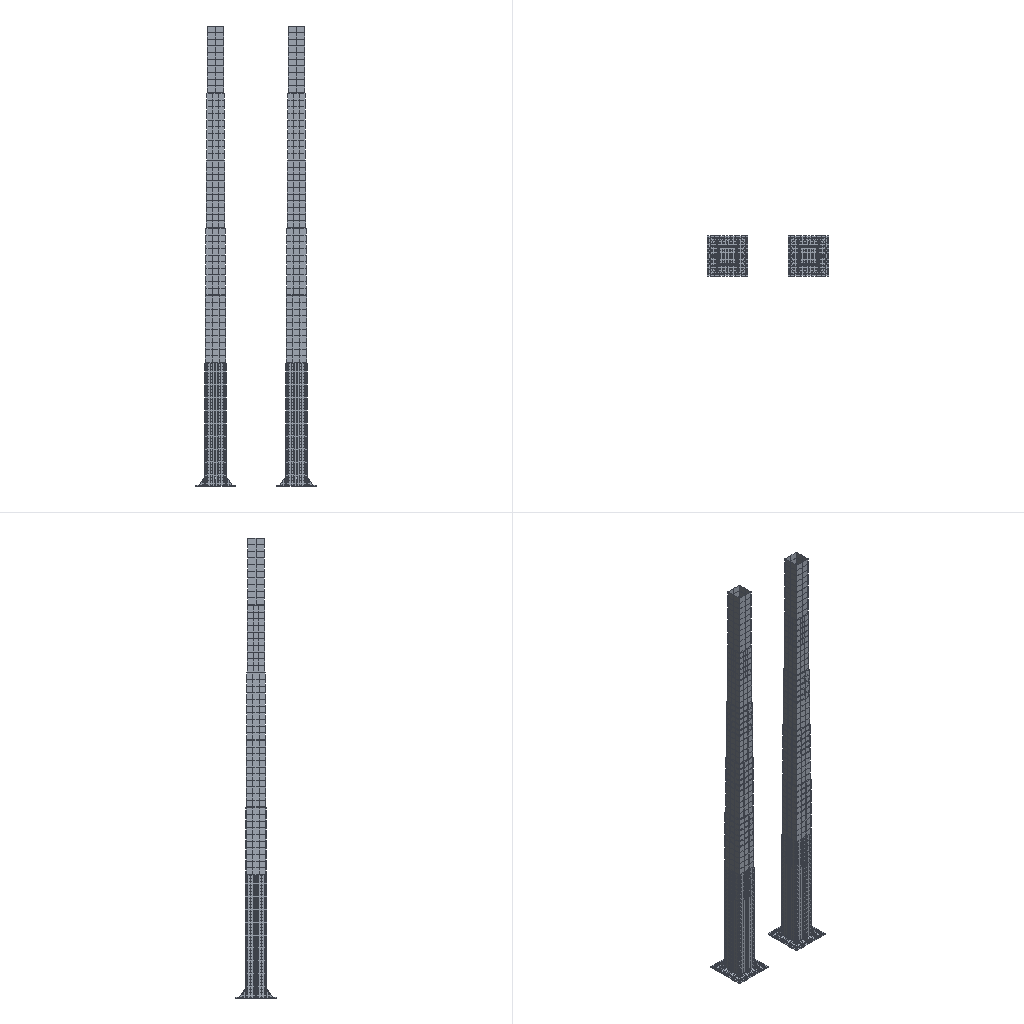Simulation study | abaqus
Set-up summary:
category,name,step,type,value,unit,region
solver,abaqus
solver,version,,,Abaqus/Standard 2020
units,not stated in the deck,,not stated
analysis,deck,,transient,transient
load_step,Step-1,Step-1,transient
load_step,requested,,,1
mesh,nodes,,,19952
mesh,elements,,,10428
element_type,C3D8R,,solid,10428
load,load commands in deck,,count,1
bc,support commands in deck,,count,1
material,MATERIAL-1,,in results
check,setup vs results,,match,"per instance, exact: element labels, types and connectivity; labels of the nodes the elements use; coordinates of those nodes at SINGLE_PRECISION in 12 of 12 instance(s)"
Abaqus input file, long lists of numbers shortened, first 444 of 2434 lines:
*Heading
** Job name: Job-1 Model name: Model-1
** Generated by: Abaqus/CAE 2020
*Preprint, echo=NO, model=NO, history=NO, contact=NO
**
** PARTS
**
*Part, name=work-1
*Node
      1,        -392.,         400.,   205.556
      2,        -400.,         400.,   205.556
** (8182 more lines like these left out)
*Element, type=C3D8R
 1,   11,    7,    8, 1147,    1,    2,    3,    4
 2, 1147,    8, 1146, 1148,    4,    3, 1079, 1078
** (4372 more lines like these left out)
*Nset, nset=Set-2, generate
    1,  8184,     1
*Elset, elset=Set-2, generate
    1,  4374,     1
** Section: Section-1
*Solid Section, elset=Set-2, material=Material-1
,
*End Part
**
*Part, name=work-2
*Node
      1,        381.5,        -379.,        3354.
      2,        381.5,         379.,        3354.
** (382 more lines like these left out)
*Element, type=C3D8R
  1,  22,  12,   1,   8,  46,  36,  25,  32
  2,  20,  14,   3,   7,  44,  38,  27,  31
** (178 more lines like these left out)
*Nset, nset=Set-1, generate
   1,  384,    1
*Elset, elset=Set-1, generate
   1,  180,    1
** Section: Section-1
*Solid Section, elset=Set-1, material=Material-1
,
*End Part
**
*Part, name=work-3
*Node
      1,        -305.,       -307.5,       13378.
      2,         305.,       -307.5,       13378.
** (254 more lines like these left out)
*Element, type=C3D8R
  1,  15,  10,   1,   8,  31,  26,  17,  24
  2,  14,  11,   3,   7,  30,  27,  19,  23
** (118 more lines like these left out)
*Nset, nset=Set-1, generate
   1,  256,    1
*Elset, elset=Set-1, generate
   1,  120,    1
** Section: Section-1
*Solid Section, elset=Set-1, material=Material-1
,
*End Part
**
*Part, name=work-4
*Node
      1,       -360.5,        -363.,        5860.
      2,        360.5,        -363.,        5860.
** (382 more lines like these left out)
*Element, type=C3D8R
  1,  22,  12,   1,   8,  46,  36,  25,  32
  2,  21,   7,   3,  11,  45,  31,  27,  35
** (178 more lines like these left out)
*Nset, nset=Set-1, generate
   1,  384,    1
*Elset, elset=Set-1, generate
   1,  180,    1
** Section: Section-1
*Solid Section, elset=Set-1, material=Material-1
,
*End Part
**
*Part, name=work-5
*Node
      1,        -342.,       -344.5,        8366.
      2,         342.,       -344.5,        8366.
** (382 more lines like these left out)
*Element, type=C3D8R
  1,  22,  12,   1,   8,  46,  36,  25,  32
  2,  21,   7,   3,  11,  45,  31,  27,  35
** (178 more lines like these left out)
*Nset, nset=Set-1, generate
   1,  384,    1
*Elset, elset=Set-1, generate
   1,  180,    1
** Section: Section-1
*Solid Section, elset=Set-1, material=Material-1
,
*End Part
**
*Part, name=work-6
*Node
      1,        323.5,        -326.,       10872.
      2,        323.5,         326.,       10872.
** (382 more lines like these left out)
*Element, type=C3D8R
  1,  22,  12,   1,   8,  46,  36,  25,  32
  2,  20,  14,   3,   7,  44,  38,  27,  31
** (178 more lines like these left out)
*Nset, nset=Set-1, generate
   1,  384,    1
*Elset, elset=Set-1, generate
   1,  180,    1
** Section: Section-1
*Solid Section, elset=Set-1, material=Material-1
,
*End Part
**
*Part, name=work-8
*Node
      1,        3342.,       -344.5,       12073.
      2,        2658.,       -344.5,       12073.
** (382 more lines like these left out)
*Element, type=C3D8R
  1,  22,  12,   1,   8,  46,  36,  25,  32
  2,  20,  14,   3,   7,  44,  38,  27,  31
** (178 more lines like these left out)
*Nset, nset=Set-1, generate
   1,  384,    1
*Elset, elset=Set-1, generate
   1,  180,    1
** Section: Section-1
*Solid Section, elset=Set-1, material=Material-1
,
*End Part
**
*Part, name=work-9
*Node
      1,       3360.5,        -363.,        9567.
      2,       2639.5,        -363.,        9567.
** (382 more lines like these left out)
*Element, type=C3D8R
  1,  22,  12,   1,   8,  46,  36,  25,  32
  2,  21,   7,   3,  11,  45,  31,  27,  35
** (178 more lines like these left out)
*Nset, nset=Set-1, generate
   1,  384,    1
*Elset, elset=Set-1, generate
   1,  180,    1
** Section: Section-1
*Solid Section, elset=Set-1, material=Material-1
,
*End Part
**
*Part, name=work-10
*Node
      1,        3305.,       -307.5,       17085.
      2,        2695.,       -307.5,       17085.
** (254 more lines like these left out)
*Element, type=C3D8R
  1,  15,  10,   1,   8,  31,  26,  17,  24
  2,  14,  11,   3,   7,  30,  27,  19,  23
** (118 more lines like these left out)
*Nset, nset=Set-1, generate
   1,  256,    1
*Elset, elset=Set-1, generate
   1,  120,    1
** Section: Section-1
*Solid Section, elset=Set-1, material=Material-1
,
*End Part
**
*Part, name=work-11
*Node
      1,       2618.5,        -379.,        7061.
      2,       2618.5,         379.,        7061.
** (382 more lines like these left out)
*Element, type=C3D8R
  1,  22,  12,   1,   8,  46,  36,  25,  32
  2,  20,  14,   3,   7,  44,  38,  27,  31
** (178 more lines like these left out)
*Nset, nset=Set-1, generate
   1,  384,    1
*Elset, elset=Set-1, generate
   1,  180,    1
** Section: Section-1
*Solid Section, elset=Set-1, material=Material-1
,
*End Part
**
*Part, name=work-12
*Node
      1,       2676.5,        -326.,       14579.
      2,       2676.5,         326.,       14579.
** (382 more lines like these left out)
*Element, type=C3D8R
  1,  22,  12,   1,   8,  46,  36,  25,  32
  2,  20,  14,   3,   7,  44,  38,  27,  31
** (178 more lines like these left out)
*Nset, nset=Set-1, generate
   1,  384,    1
*Elset, elset=Set-1, generate
   1,  180,    1
** Section: Section-1
*Solid Section, elset=Set-1, material=Material-1
,
*End Part
**
**
** ASSEMBLY
**
*Assembly, name=Assembly
**
*Instance, name=work-1-1, part=work-1
*End Instance
**
*Instance, name=work-2-1, part=work-2
*End Instance
**
*Instance, name=work-3-1, part=work-3
*End Instance
**
*Instance, name=work-4-1, part=work-4
*End Instance
**
*Instance, name=work-5-1, part=work-5
*End Instance
**
*Instance, name=work-6-1, part=work-6
*End Instance
**
*Instance, name=work-8-1, part=work-8
*End Instance
**
*Instance, name=work-9-1, part=work-9
*End Instance
**
*Instance, name=work-10-1, part=work-10
*End Instance
**
*Instance, name=work-11-1, part=work-11
*End Instance
**
*Instance, name=work-12-1, part=work-12
*End Instance
**
*Instance, name=work-1-1-lin-2-1, part=work-1
       3000.,           0.,           0.
*End Instance
**
*Node
      1,        3000.,          55.,           0.
*Node
      2,        1500.,          55.,           0.
*Nset, nset=Set-2
 2,
*Nset, nset=m_Set-1
 2,
*Elset, elset=_load_S3, internal, instance=work-8-1, generate
   9,  117,   12
*Elset, elset=_load_S3, internal, instance=work-9-1, generate
  10,  118,   12
*Elset, elset=_load_S3, internal, instance=work-4-1, generate
  70,  178,   12
*Elset, elset=_load_S4, internal, instance=work-8-1, generate
   2,  110,   12
*Elset, elset=_load_S4, internal, instance=work-9-1, generate
   3,  111,   12
*Elset, elset=_load_S4, internal, instance=work-4-1, generate
  63,  171,   12
*Elset, elset=_load_S4, internal, instance=work-10-1, generate
  2,  74,   8
*Elset, elset=_load_S4, internal, instance=work-5-1, generate
  63,  171,   12
*Elset, elset=_load_S4, internal, instance=work-3-1, generate
  42,  114,    8
*Elset, elset=_load_S5, internal, instance=work-8-1, generate
  10,  118,   12
*Elset, elset=_load_S5, internal, instance=work-9-1, generate
  11,  119,   12
*Elset, elset=_load_S5, internal, instance=work-4-1, generate
  71,  179,   12
*Elset, elset=_load_S5, internal, instance=work-10-1, generate
  3,  75,   8
*Elset, elset=_load_S5, internal, instance=work-5-1
  64,  71,  76,  83,  88,  95, 100, 107, 112, 119, 124, 131, 136, 143, 148, 155
 160, 167, 172, 179
*Elset, elset=_load_S5, internal, instance=work-3-1, generate
  43,  115,    8
*Surface, type=ELEMENT, name=load
_load_S3, S3
_load_S4, S4
_load_S5, S5
*Elset, elset=_m_Surf-2_S1, internal, instance=work-1-1
  569,  570,  571,  572,  573,  574,  575,  576,  577,  578,  579,  580,  581,  582,  583,  584
  585,  586,  587,  588,  589,  590,  591,  592,  593,  594,  595,  596,  597,  598,  599,  600
** (19 more lines like these left out)
*Elset, elset=_m_Surf-2_S1, internal, instance=work-1-1-lin-2-1
  569,  570,  571,  572,  573,  574,  575,  576,  577,  578,  579,  580,  581,  582,  583,  584
  585,  586,  587,  588,  589,  590,  591,  592,  593,  594,  595,  596,  597,  598,  599,  600
** (19 more lines like these left out)
*Elset, elset=_m_Surf-2_S4, internal, instance=work-1-1
  137,  138,  139,  140,  141,  142,  143,  144,  145,  146,  147,  148,  149,  150,  151,  152
  153,  154,  155,  156,  157,  158,  159,  160,  161,  162,  163,  164,  165,  166,  167,  168
** (101 more lines like these left out)
*Elset, elset=_m_Surf-2_S4, internal, instance=work-1-1-lin-2-1
  137,  138,  139,  140,  141,  142,  143,  144,  145,  146,  147,  148,  149,  150,  151,  152
  153,  154,  155,  156,  157,  158,  159,  160,  161,  162,  163,  164,  165,  166,  167,  168
** (101 more lines like these left out)
*Elset, elset=_m_Surf-2_S2, internal, instance=work-1-1
 281, 282, 283, 284, 285, 286, 287, 288, 289, 290, 291, 292, 293, 294, 295, 296
 297, 298, 299, 300, 301, 302, 303, 304, 305, 306, 307, 308, 309, 310, 311, 312
** (5 more lines like these left out)
*Elset, elset=_m_Surf-2_S2, internal, instance=work-1-1-lin-2-1
 281, 282, 283, 284, 285, 286, 287, 288, 289, 290, 291, 292, 293, 294, 295, 296
 297, 298, 299, 300, 301, 302, 303, 304, 305, 306, 307, 308, 309, 310, 311, 312
** (5 more lines like these left out)
*Elset, elset=_m_Surf-2_S5, internal, instance=work-1-1
 2081, 2082, 2083, 2084, 2085, 2086, 2087, 2088, 2089, 2090, 2091, 2092, 2093, 2094, 2095, 2096
 2097, 2098, 2099, 2100, 2101, 2102, 2103, 2104, 2105, 2106, 2107, 2108, 2109, 2110, 2111, 2112
** (3 more lines like these left out)
*Elset, elset=_m_Surf-2_S5, internal, instance=work-1-1-lin-2-1
 2081, 2082, 2083, 2084, 2085, 2086, 2087, 2088, 2089, 2090, 2091, 2092, 2093, 2094, 2095, 2096
 2097, 2098, 2099, 2100, 2101, 2102, 2103, 2104, 2105, 2106, 2107, 2108, 2109, 2110, 2111, 2112
** (3 more lines like these left out)
*Elset, elset=_m_Surf-2_S3, internal, instance=work-1-1
 2153, 2154, 2155, 2156, 2157, 2158, 2159, 2160, 2161, 2162, 2163, 2164, 2165, 2166, 2167, 2168
 2169, 2170, 2171, 2172, 2173, 2174, 2175, 2176, 2177, 2178, 2179, 2180, 2181, 2182, 2183, 2184
** (3 more lines like these left out)
*Elset, elset=_m_Surf-2_S3, internal, instance=work-1-1-lin-2-1
 2153, 2154, 2155, 2156, 2157, 2158, 2159, 2160, 2161, 2162, 2163, 2164, 2165, 2166, 2167, 2168
 2169, 2170, 2171, 2172, 2173, 2174, 2175, 2176, 2177, 2178, 2179, 2180, 2181, 2182, 2183, 2184
** (3 more lines like these left out)
*Surface, type=ELEMENT, name=m_Surf-2
_m_Surf-2_S1, S1
_m_Surf-2_S4, S4
_m_Surf-2_S2, S2
_m_Surf-2_S5, S5
_m_Surf-2_S3, S3
*Elset, elset=_m_Surf-8_S6, internal, instance=work-6-1
   1,   2,   3,  13,  14,  15,  25,  26,  27,  37,  38,  39,  49,  50,  51,  61
  62,  63,  73,  74,  75,  85,  86,  87,  97,  98,  99, 109, 110, 111, 121, 122
** (1 more lines like these left out)
*Elset, elset=_m_Surf-8_S6, internal, instance=work-12-1
   1,   2,   4,  12,  13,  14,  16,  24,  25,  26,  28,  36,  37,  38,  40,  48
  49,  50,  52,  60,  61,  62,  64,  72,  73,  74,  76,  84,  85,  86,  88,  96
** (2 more lines like these left out)
*Elset, elset=_m_Surf-8_S5, internal, instance=work-6-1
   5,   6,   8,  10,  17,  18,  20,  22,  29,  30,  32,  34,  41,  42,  44,  46
  53,  54,  56,  58,  65,  66,  68,  70,  77,  78,  80,  82,  89,  90,  92,  94
** (2 more lines like these left out)
*Elset, elset=_m_Surf-8_S5, internal, instance=work-12-1
   6,   8,  18,  20,  30,  32,  42,  44,  54,  56,  66,  68,  78,  80,  90,  92
 102, 104, 114, 116, 126, 128, 138, 140, 150, 152, 162, 164, 174, 176
*Elset, elset=_m_Surf-8_S3, internal, instance=work-6-1
   7,   9,  11,  12,  19,  21,  23,  24,  31,  33,  35,  36,  43,  45,  47,  48
  55,  57,  59,  60,  67,  69,  71,  72,  79,  81,  83,  84,  91,  93,  95,  96
** (2 more lines like these left out)
*Elset, elset=_m_Surf-8_S3, internal, instance=work-12-1
   3,   5,   7,   9,  10,  11,  15,  17,  19,  21,  22,  23,  27,  29,  31,  33
  34,  35,  39,  41,  43,  45,  46,  47,  51,  53,  55,  57,  58,  59,  63,  65
** (4 more lines like these left out)
*Elset, elset=_m_Surf-8_S4, internal, instance=work-6-1, generate
   4,  172,   12
*Surface, type=ELEMENT, name=m_Surf-8
_m_Surf-8_S6, S6
_m_Surf-8_S5, S5
_m_Surf-8_S4, S4
_m_Surf-8_S3, S3
*Elset, elset=_m_Surf-11_S6, internal, instance=work-4-1
   1,   3,   4,   5,  13,  15,  16,  17,  25,  27,  28,  29,  37,  39,  40,  41
  49,  51,  52,  53,  61,  63,  64,  65,  73,  75,  76,  77,  85,  87,  88,  89
** (2 more lines like these left out)
*Elset, elset=_m_Surf-11_S6, internal, instance=work-9-1
   1,   3,   4,   5,  13,  15,  16,  17,  25,  27,  28,  29,  37,  39,  40,  41
  49,  51,  52,  53,  61,  63,  64,  65,  73,  75,  76,  77,  85,  87,  88,  89
** (2 more lines like these left out)
*Elset, elset=_m_Surf-11_S5, internal, instance=work-4-1
   6,   7,  10,  18,  19,  22,  30,  31,  34,  42,  43,  46,  54,  55,  58,  66
  67,  70,  78,  79,  82,  90,  91,  94, 102, 103, 106, 114, 115, 118, 126, 127
** (1 more lines like these left out)
*Elset, elset=_m_Surf-11_S5, internal, instance=work-9-1
   6,   7,  10,  18,  19,  22,  30,  31,  34,  42,  43,  46,  54,  55,  58,  66
  67,  70,  78,  79,  82,  90,  91,  94, 102, 103, 106, 114, 115, 118, 126, 127
** (1 more lines like these left out)
*Elset, elset=_m_Surf-11_S3, internal, instance=work-4-1
   2,   8,   9,  11,  12,  14,  20,  21,  23,  24,  26,  32,  33,  35,  36,  38
  44,  45,  47,  48,  50,  56,  57,  59,  60,  62,  68,  69,  71,  72,  74,  80
** (3 more lines like these left out)
*Elset, elset=_m_Surf-11_S3, internal, instance=work-9-1
   2,   8,   9,  11,  12,  14,  20,  21,  23,  24,  26,  32,  33,  35,  36,  38
  44,  45,  47,  48,  50,  56,  57,  59,  60,  62,  68,  69,  71,  72,  74,  80
** (3 more lines like these left out)
*Surface, type=ELEMENT, name=m_Surf-11
_m_Surf-11_S6, S6
_m_Surf-11_S5, S5
_m_Surf-11_S3, S3
*Elset, elset=_s_Surf-1_S4, internal, instance=work-1-1
 2448, 2457, 2461, 2470, 2481, 2493, 2497, 2506, 2513, 2514, 2515, 2519, 2533, 2537, 2543, 2561
 2564, 2573, 2576, 2579, 2584, 2657, 2669, 2671, 2673, 2675, 2679, 2687, 2689, 2691, 2693, 2705
** (27 more lines like these left out)
*Elset, elset=_s_Surf-1_S4, internal, instance=work-1-1-lin-2-1
 2448, 2457, 2461, 2470, 2481, 2493, 2497, 2506, 2513, 2514, 2515, 2519, 2533, 2537, 2543, 2561
 2564, 2573, 2576, 2579, 2584, 2657, 2669, 2671, 2673, 2675, 2679, 2687, 2689, 2691, 2693, 2705
** (27 more lines like these left out)
*Elset, elset=_s_Surf-1_S3, internal, instance=work-1-1
 2445, 2450, 2460, 2467, 2472, 2480, 2484, 2487, 2496, 2503, 2508, 2512, 2518, 2536, 2544, 2562
 2574, 2583, 2594, 2595, 2598, 2599, 2654, 2659, 2662, 2663, 2676, 2680, 2702, 2707, 2711, 2716
** (10 more lines like these left out)
*Elset, elset=_s_Surf-1_S3, internal, instance=work-1-1-lin-2-1
 2445, 2450, 2460, 2467, 2472, 2480, 2484, 2487, 2496, 2503, 2508, 2512, 2518, 2536, 2544, 2562
 2574, 2583, 2594, 2595, 2598, 2599, 2654, 2659, 2662, 2663, 2676, 2680, 2702, 2707, 2711, 2716
** (10 more lines like these left out)
*Elset, elset=_s_Surf-1_S2, internal, instance=work-1-1
 2451, 2452, 2453, 2463, 2464, 2473, 2474, 2475, 2488, 2499, 2500, 2521, 2522, 2539, 2540, 2547
 2548, 2549, 2550, 2551, 2566, 2567, 2585, 2682, 2683, 2694, 2695, 2696, 2697, 2712, 2713, 2821
** (6 more lines like these left out)
*Elset, elset=_s_Surf-1_S2, internal, instance=work-1-1-lin-2-1
 2451, 2452, 2453, 2463, 2464, 2473, 2474, 2475, 2488, 2499, 2500, 2521, 2522, 2539, 2540, 2547
 2548, 2549, 2550, 2551, 2566, 2567, 2585, 2682, 2683, 2694, 2695, 2696, 2697, 2712, 2713, 2821
** (6 more lines like these left out)
*Elset, elset=_s_Surf-1_S1, internal, instance=work-1-1
 2529, 2530, 2531, 2532, 2590, 2591, 2592, 2593, 3663, 3664, 3665, 3666, 3734, 3735, 3736, 3737
 3740, 3741, 3746, 3747, 3748, 3749, 3910, 3911, 3994, 3995, 4000, 4001, 4002, 4003, 4013, 4014
** (1 more lines like these left out)
*Elset, elset=_s_Surf-1_S1, internal, instance=work-1-1-lin-2-1
 2529, 2530, 2531, 2532, 2590, 2591, 2592, 2593, 3663, 3664, 3665, 3666, 3734, 3735, 3736, 3737
 3740, 3741, 3746, 3747, 3748, 3749, 3910, 3911, 3994, 3995, 4000, 4001, 4002, 4003, 4013, 4014
** (1 more lines like these left out)
*Elset, elset=_s_Surf-1_S6, internal, instance=work-1-1
 2489, 2491, 2602, 2604, 2606, 2608, 2610, 2612, 2614, 2616, 2618, 2620, 2622, 2624, 2626, 2628
 2630, 2632, 2634, 2636, 2638, 2640, 2642, 2644, 2646, 2648, 2650, 2652, 2802, 2804, 2806, 2808
** (7 more lines like these left out)
*Elset, elset=_s_Surf-1_S6, internal, instance=work-1-1-lin-2-1
 2489, 2491, 2602, 2604, 2606, 2608, 2610, 2612, 2614, 2616, 2618, 2620, 2622, 2624, 2626, 2628
 2630, 2632, 2634, 2636, 2638, 2640, 2642, 2644, 2646, 2648, 2650, 2652, 2802, 2804, 2806, 2808
** (7 more lines like these left out)
*Elset, elset=_s_Surf-1_S5, internal, instance=work-1-1
 2799, 2801, 2895, 2897, 3777, 3779, 3797, 3799, 3945, 3947, 3965, 3967, 4276, 4278, 4342
*Elset, elset=_s_Surf-1_S5, internal, instance=work-1-1-lin-2-1
 2799, 2801, 2895, 2897, 3777, 3779, 3797, 3799, 3945, 3947, 3965, 3967, 4276, 4278, 4342
*Surface, type=ELEMENT, name=s_Surf-1
_s_Surf-1_S4, S4
_s_Surf-1_S3, S3
_s_Surf-1_S2, S2
_s_Surf-1_S6, S6
_s_Surf-1_S1, S1
Last 724 lines:
 3840, 3842, 3843
*Elset, elset=__Int-1_gcs0_2778_S3, internal, instance=work-1-1-lin-2-1
 3841,
*Surface, type=ELEMENT, name=_Int-1_gcs0_2778, internal
__Int-1_gcs0_2778_S4, S4
__Int-1_gcs0_2778_S3, S3
*Elset, elset=__Int-1_gcs0_2779_S4, internal, instance=work-1-1-lin-2-1
 3616, 3619
*Elset, elset=__Int-1_gcs0_2779_S3, internal, instance=work-1-1-lin-2-1
 3617,
*Elset, elset=__Int-1_gcs0_2779_S2, internal, instance=work-1-1-lin-2-1
 3620,
*Surface, type=ELEMENT, name=_Int-1_gcs0_2779, internal
__Int-1_gcs0_2779_S4, S4
__Int-1_gcs0_2779_S3, S3
__Int-1_gcs0_2779_S2, S2
*Elset, elset=__Int-1_gcs0_2780_S4, internal, instance=work-1-1-lin-2-1
 4075,
*Elset, elset=__Int-1_gcs0_2780_S3, internal, instance=work-1-1-lin-2-1
 4076, 4079
*Elset, elset=__Int-1_gcs0_2780_S2, internal, instance=work-1-1-lin-2-1
 4081,
*Surface, type=ELEMENT, name=_Int-1_gcs0_2780, internal
__Int-1_gcs0_2780_S4, S4
__Int-1_gcs0_2780_S3, S3
__Int-1_gcs0_2780_S2, S2
*Elset, elset=__Int-1_gcs0_2781_S4, internal, instance=work-1-1-lin-2-1
 4063, 4069
*Elset, elset=__Int-1_gcs0_2781_S3, internal, instance=work-1-1-lin-2-1
 4066, 4071
*Surface, type=ELEMENT, name=_Int-1_gcs0_2781, internal
__Int-1_gcs0_2781_S4, S4
__Int-1_gcs0_2781_S3, S3
*Elset, elset=__Int-1_gcs0_2788_S4, internal, instance=work-1-1-lin-2-1
 4051,
*Elset, elset=__Int-1_gcs0_2788_S3, internal, instance=work-1-1-lin-2-1
 4052, 4053
*Elset, elset=__Int-1_gcs0_2788_S2, internal, instance=work-1-1-lin-2-1
 4056,
*Surface, type=ELEMENT, name=_Int-1_gcs0_2788, internal
__Int-1_gcs0_2788_S4, S4
__Int-1_gcs0_2788_S3, S3
__Int-1_gcs0_2788_S2, S2
*Elset, elset=__Int-1_gcs0_2790_S3, internal, instance=work-1-1-lin-2-1
 3633,
*Elset, elset=__Int-1_gcs0_2790_S4, internal, instance=work-1-1-lin-2-1
 3634,
*Elset, elset=__Int-1_gcs0_2790_S2, internal, instance=work-1-1-lin-2-1
 3637, 3638
*Surface, type=ELEMENT, name=_Int-1_gcs0_2790, internal
__Int-1_gcs0_2790_S3, S3
__Int-1_gcs0_2790_S4, S4
__Int-1_gcs0_2790_S2, S2
*Elset, elset=__Int-1_gcs0_2792_S3, internal, instance=work-1-1-lin-2-1
 3868, 3870
*Elset, elset=__Int-1_gcs0_2792_S4, internal, instance=work-1-1-lin-2-1
 3869,
*Elset, elset=__Int-1_gcs0_2792_S2, internal, instance=work-1-1-lin-2-1
 3873,
*Surface, type=ELEMENT, name=_Int-1_gcs0_2792, internal
__Int-1_gcs0_2792_S3, S3
__Int-1_gcs0_2792_S4, S4
__Int-1_gcs0_2792_S2, S2
*Elset, elset=__Int-1_gcs0_2794_S4, internal, instance=work-1-1-lin-2-1
 3582, 3585, 3587
*Elset, elset=__Int-1_gcs0_2794_S3, internal, instance=work-1-1-lin-2-1
 3583,
*Surface, type=ELEMENT, name=_Int-1_gcs0_2794, internal
__Int-1_gcs0_2794_S4, S4
__Int-1_gcs0_2794_S3, S3
*Elset, elset=__Int-1_gcs0_2889_S4, internal, instance=work-1-1-lin-2-1
 4170, 4173
*Elset, elset=__Int-1_gcs0_2889_S3, internal, instance=work-1-1-lin-2-1
 4171, 4174
*Surface, type=ELEMENT, name=_Int-1_gcs0_2889, internal
__Int-1_gcs0_2889_S4, S4
__Int-1_gcs0_2889_S3, S3
*Elset, elset=__Int-1_gcs0_2891_S4, internal, instance=work-1-1-lin-2-1
 3826, 3829
*Elset, elset=__Int-1_gcs0_2891_S3, internal, instance=work-1-1-lin-2-1
 3827,
*Elset, elset=__Int-1_gcs0_2891_S2, internal, instance=work-1-1-lin-2-1
 3830,
*Surface, type=ELEMENT, name=_Int-1_gcs0_2891, internal
__Int-1_gcs0_2891_S4, S4
__Int-1_gcs0_2891_S3, S3
__Int-1_gcs0_2891_S2, S2
*Elset, elset=__Int-1_gcs0_2892_S3, internal, instance=work-1-1-lin-2-1
 2471,
*Elset, elset=__Int-1_gcs0_2892_S4, internal, instance=work-1-1-lin-2-1, generate
 2472,  2478,     3
*Surface, type=ELEMENT, name=_Int-1_gcs0_2892, internal
__Int-1_gcs0_2892_S3, S3
__Int-1_gcs0_2892_S4, S4
*Elset, elset=__Int-1_gcs0_2893_S4, internal, instance=work-1-1-lin-2-1
 4186, 4191, 4192
*Elset, elset=__Int-1_gcs0_2893_S3, internal, instance=work-1-1-lin-2-1
 4187,
*Surface, type=ELEMENT, name=_Int-1_gcs0_2893, internal
__Int-1_gcs0_2893_S4, S4
__Int-1_gcs0_2893_S3, S3
*Elset, elset=__Int-1_gcs0_2895_S3, internal, instance=work-1-1-lin-2-1
 3926,
*Elset, elset=__Int-1_gcs0_2895_S4, internal, instance=work-1-1-lin-2-1, generate
 3927,  3933,     3
*Surface, type=ELEMENT, name=_Int-1_gcs0_2895, internal
__Int-1_gcs0_2895_S3, S3
__Int-1_gcs0_2895_S4, S4
*Elset, elset=__Int-1_gcs0_2896_S2, internal, instance=work-1-1-lin-2-1, generate
 2503,  2506,     1
*Surface, type=ELEMENT, name=_Int-1_gcs0_2896, internal
__Int-1_gcs0_2896_S2, S2
*Elset, elset=__Int-1_gcs0_2897_S3, internal, instance=work-1-1-lin-2-1
 3679,
*Elset, elset=__Int-1_gcs0_2897_S4, internal, instance=work-1-1-lin-2-1
 3680,
*Elset, elset=__Int-1_gcs0_2897_S2, internal, instance=work-1-1-lin-2-1
 3681, 3682
*Surface, type=ELEMENT, name=_Int-1_gcs0_2897, internal
__Int-1_gcs0_2897_S3, S3
__Int-1_gcs0_2897_S4, S4
__Int-1_gcs0_2897_S2, S2
*Elset, elset=__Int-1_gcs0_2898_S4, internal, instance=work-1-1-lin-2-1
 3814, 3817, 3819
*Elset, elset=__Int-1_gcs0_2898_S3, internal, instance=work-1-1-lin-2-1
 3815,
*Surface, type=ELEMENT, name=_Int-1_gcs0_2898, internal
__Int-1_gcs0_2898_S4, S4
__Int-1_gcs0_2898_S3, S3
*Elset, elset=__Int-1_gcs0_2903_S3, internal, instance=work-1-1-lin-2-1
 2519, 2521
*Elset, elset=__Int-1_gcs0_2903_S4, internal, instance=work-1-1-lin-2-1
 2520,
*Elset, elset=__Int-1_gcs0_2903_S2, internal, instance=work-1-1-lin-2-1
 2523,
*Surface, type=ELEMENT, name=_Int-1_gcs0_2903, internal
__Int-1_gcs0_2903_S3, S3
__Int-1_gcs0_2903_S4, S4
__Int-1_gcs0_2903_S2, S2
*Elset, elset=__Int-1_gcs0_2907_S4, internal, instance=work-1-1-lin-2-1
 4175,
*Elset, elset=__Int-1_gcs0_2907_S3, internal, instance=work-1-1-lin-2-1
 4176,
*Elset, elset=__Int-1_gcs0_2907_S2, internal, instance=work-1-1-lin-2-1
 4179, 4180
*Surface, type=ELEMENT, name=_Int-1_gcs0_2907, internal
__Int-1_gcs0_2907_S4, S4
__Int-1_gcs0_2907_S3, S3
__Int-1_gcs0_2907_S2, S2
*Elset, elset=__Int-1_gcs0_2909_S3, internal, instance=work-1-1-lin-2-1
 2481, 2488
*Elset, elset=__Int-1_gcs0_2909_S4, internal, instance=work-1-1-lin-2-1
 2482, 2486
*Surface, type=ELEMENT, name=_Int-1_gcs0_2909, internal
__Int-1_gcs0_2909_S3, S3
__Int-1_gcs0_2909_S4, S4
*Elset, elset=__Int-1_gcs0_2912_S4, internal, instance=work-1-1-lin-2-1
 2499, 2501
*Elset, elset=__Int-1_gcs0_2912_S3, internal, instance=work-1-1-lin-2-1
 2500,
*Elset, elset=__Int-1_gcs0_2912_S2, internal, instance=work-1-1-lin-2-1
 2502,
*Surface, type=ELEMENT, name=_Int-1_gcs0_2912, internal
__Int-1_gcs0_2912_S4, S4
__Int-1_gcs0_2912_S3, S3
__Int-1_gcs0_2912_S2, S2
*Elset, elset=__Int-1_gcs0_2919_S4, internal, instance=work-1-1-lin-2-1
 3972, 3976, 3977
*Elset, elset=__Int-1_gcs0_2919_S3, internal, instance=work-1-1-lin-2-1
 3973,
*Surface, type=ELEMENT, name=_Int-1_gcs0_2919, internal
__Int-1_gcs0_2919_S4, S4
__Int-1_gcs0_2919_S3, S3
*Elset, elset=__Int-1_gcs0_2921_S4, internal, instance=work-1-1-lin-2-1
 2544, 2551, 2556
*Elset, elset=__Int-1_gcs0_2921_S3, internal, instance=work-1-1-lin-2-1
 2545,
*Surface, type=ELEMENT, name=_Int-1_gcs0_2921, internal
__Int-1_gcs0_2921_S4, S4
__Int-1_gcs0_2921_S3, S3
*Elset, elset=__Int-1_gcs0_2923_S4, internal, instance=work-1-1-lin-2-1
 4259,
*Elset, elset=__Int-1_gcs0_2923_S3, internal, instance=work-1-1-lin-2-1
 4260,
*Elset, elset=__Int-1_gcs0_2923_S2, internal, instance=work-1-1-lin-2-1
 4261, 4262
*Surface, type=ELEMENT, name=_Int-1_gcs0_2923, internal
__Int-1_gcs0_2923_S4, S4
__Int-1_gcs0_2923_S3, S3
__Int-1_gcs0_2923_S2, S2
*Elset, elset=__Int-1_gcs0_2925_S2, internal, instance=work-1-1-lin-2-1, generate
 2572,  2575,     1
*Surface, type=ELEMENT, name=_Int-1_gcs0_2925, internal
__Int-1_gcs0_2925_S2, S2
*Elset, elset=__Int-1_gcs0_3325_S4, internal, instance=work-1-1-lin-2-1
 4307,
*Elset, elset=__Int-1_gcs0_3325_S3, internal, instance=work-1-1-lin-2-1
 4308,
*Elset, elset=__Int-1_gcs0_3325_S2, internal, instance=work-1-1-lin-2-1
 4311, 4312
*Surface, type=ELEMENT, name=_Int-1_gcs0_3325, internal
__Int-1_gcs0_3325_S4, S4
__Int-1_gcs0_3325_S3, S3
__Int-1_gcs0_3325_S2, S2
*Elset, elset=__Int-1_gcs0_3326_S4, internal, instance=work-1-1-lin-2-1
 2549, 2554
*Elset, elset=__Int-1_gcs0_3326_S3, internal, instance=work-1-1-lin-2-1
 2550,
*Elset, elset=__Int-1_gcs0_3326_S2, internal, instance=work-1-1-lin-2-1
 2555,
*Surface, type=ELEMENT, name=_Int-1_gcs0_3326, internal
__Int-1_gcs0_3326_S4, S4
__Int-1_gcs0_3326_S3, S3
__Int-1_gcs0_3326_S2, S2
*Elset, elset=__Int-1_gcs0_3327_S3, internal, instance=work-1-1-lin-2-1
 4293,
*Elset, elset=__Int-1_gcs0_3327_S4, internal, instance=work-1-1-lin-2-1
 4294,
*Elset, elset=__Int-1_gcs0_3327_S2, internal, instance=work-1-1-lin-2-1
 4295, 4296
*Surface, type=ELEMENT, name=_Int-1_gcs0_3327, internal
__Int-1_gcs0_3327_S3, S3
__Int-1_gcs0_3327_S4, S4
__Int-1_gcs0_3327_S2, S2
*Elset, elset=__Int-1_gcs0_3328_S3, internal, instance=work-1-1-lin-2-1
 2507, 2509, 2514
*Elset, elset=__Int-1_gcs0_3328_S4, internal, instance=work-1-1-lin-2-1
 2508,
*Surface, type=ELEMENT, name=_Int-1_gcs0_3328, internal
__Int-1_gcs0_3328_S3, S3
__Int-1_gcs0_3328_S4, S4
*Elset, elset=__Int-1_gcs0_3329_S3, internal, instance=work-1-1-lin-2-1
 4279,
*Elset, elset=__Int-1_gcs0_3329_S4, internal, instance=work-1-1-lin-2-1
 4280,
*Elset, elset=__Int-1_gcs0_3329_S2, internal, instance=work-1-1-lin-2-1
 4283, 4284
*Surface, type=ELEMENT, name=_Int-1_gcs0_3329, internal
__Int-1_gcs0_3329_S3, S3
__Int-1_gcs0_3329_S4, S4
__Int-1_gcs0_3329_S2, S2
*Elset, elset=__Int-1_gcs0_3330_S3, internal, instance=work-1-1-lin-2-1
 3824,
*Elset, elset=__Int-1_gcs0_3330_S4, internal, instance=work-1-1-lin-2-1, generate
 3825,  3831,     3
*Surface, type=ELEMENT, name=_Int-1_gcs0_3330, internal
__Int-1_gcs0_3330_S3, S3
__Int-1_gcs0_3330_S4, S4
*Elset, elset=__Int-1_gcs0_3331_S2, internal, instance=work-1-1-lin-2-1, generate
 3695,  3698,     1
*Surface, type=ELEMENT, name=_Int-1_gcs0_3331, internal
__Int-1_gcs0_3331_S2, S2
*Elset, elset=__Int-1_gcs0_3332_S4, internal, instance=work-1-1-lin-2-1
 4126, 4129
*Elset, elset=__Int-1_gcs0_3332_S3, internal, instance=work-1-1-lin-2-1
 4127,
*Elset, elset=__Int-1_gcs0_3332_S2, internal, instance=work-1-1-lin-2-1
 4130,
*Surface, type=ELEMENT, name=_Int-1_gcs0_3332, internal
__Int-1_gcs0_3332_S4, S4
__Int-1_gcs0_3332_S3, S3
__Int-1_gcs0_3332_S2, S2
*Elset, elset=__Int-1_gcs0_3333_S4, internal, instance=work-1-1-lin-2-1
 4143, 4146, 4148
*Elset, elset=__Int-1_gcs0_3333_S3, internal, instance=work-1-1-lin-2-1
 4144,
*Surface, type=ELEMENT, name=_Int-1_gcs0_3333, internal
__Int-1_gcs0_3333_S4, S4
__Int-1_gcs0_3333_S3, S3
*Elset, elset=__Int-1_gcs0_3334_S4, internal, instance=work-1-1-lin-2-1
 3300,
*Elset, elset=__Int-1_gcs0_3334_S3, internal, instance=work-1-1-lin-2-1
 3301, 3303
*Elset, elset=__Int-1_gcs0_3334_S2, internal, instance=work-1-1-lin-2-1
 3305,
*Surface, type=ELEMENT, name=_Int-1_gcs0_3334, internal
__Int-1_gcs0_3334_S4, S4
__Int-1_gcs0_3334_S3, S3
__Int-1_gcs0_3334_S2, S2
*Elset, elset=__Int-1_gcs0_3335_S3, internal, instance=work-1-1-lin-2-1
 2940,
*Elset, elset=__Int-1_gcs0_3335_S4, internal, instance=work-1-1-lin-2-1, generate
 2941,  2945,     2
*Surface, type=ELEMENT, name=_Int-1_gcs0_3335, internal
__Int-1_gcs0_3335_S3, S3
__Int-1_gcs0_3335_S4, S4
*Elset, elset=__Int-1_gcs0_3336_S4, internal, instance=work-1-1-lin-2-1
 4153, 4159, 4161
*Elset, elset=__Int-1_gcs0_3336_S3, internal, instance=work-1-1-lin-2-1
 4156,
*Surface, type=ELEMENT, name=_Int-1_gcs0_3336, internal
__Int-1_gcs0_3336_S4, S4
__Int-1_gcs0_3336_S3, S3
*Elset, elset=__Int-1_gcs0_3337_S2, internal, instance=work-1-1-lin-2-1, generate
 4163,  4166,     1
*Surface, type=ELEMENT, name=_Int-1_gcs0_3337, internal
__Int-1_gcs0_3337_S2, S2
*Elset, elset=__Int-1_gcs0_3338_S3, internal, instance=work-1-1-lin-2-1
 3752, 3758
*Elset, elset=__Int-1_gcs0_3338_S4, internal, instance=work-1-1-lin-2-1
 3753,
*Elset, elset=__Int-1_gcs0_3338_S2, internal, instance=work-1-1-lin-2-1
 3759,
*Surface, type=ELEMENT, name=_Int-1_gcs0_3338, internal
__Int-1_gcs0_3338_S3, S3
__Int-1_gcs0_3338_S4, S4
__Int-1_gcs0_3338_S2, S2
*Elset, elset=__Int-1_gcs0_3339_S3, internal, instance=work-1-1-lin-2-1
 3836,
*Elset, elset=__Int-1_gcs0_3339_S4, internal, instance=work-1-1-lin-2-1
 3837,
*Elset, elset=__Int-1_gcs0_3339_S2, internal, instance=work-1-1-lin-2-1
 3838, 3839
*Surface, type=ELEMENT, name=_Int-1_gcs0_3339, internal
__Int-1_gcs0_3339_S3, S3
__Int-1_gcs0_3339_S4, S4
__Int-1_gcs0_3339_S2, S2
*Elset, elset=__Int-1_gcs0_3340_S2, internal, instance=work-1-1-lin-2-1, generate
 3599,  3602,     1
*Surface, type=ELEMENT, name=_Int-1_gcs0_3340, internal
__Int-1_gcs0_3340_S2, S2
*Elset, elset=__Int-1_gcs0_3341_S3, internal, instance=work-1-1-lin-2-1
 3578, 3584
*Elset, elset=__Int-1_gcs0_3341_S4, internal, instance=work-1-1-lin-2-1
 3579,
*Elset, elset=__Int-1_gcs0_3341_S2, internal, instance=work-1-1-lin-2-1
 3586,
*Surface, type=ELEMENT, name=_Int-1_gcs0_3341, internal
__Int-1_gcs0_3341_S3, S3
__Int-1_gcs0_3341_S4, S4
__Int-1_gcs0_3341_S2, S2
*Elset, elset=__Int-1_gcs0_3342_S3, internal, instance=work-1-1-lin-2-1
 3938, 3940
*Elset, elset=__Int-1_gcs0_3342_S4, internal, instance=work-1-1-lin-2-1
 3939,
*Elset, elset=__Int-1_gcs0_3342_S2, internal, instance=work-1-1-lin-2-1
 3942,
*Surface, type=ELEMENT, name=_Int-1_gcs0_3342, internal
__Int-1_gcs0_3342_S3, S3
__Int-1_gcs0_3342_S4, S4
__Int-1_gcs0_3342_S2, S2
*Elset, elset=__Int-1_gcs0_3343_S3, internal, instance=work-1-1-lin-2-1
 3542, 3548
*Elset, elset=__Int-1_gcs0_3343_S4, internal, instance=work-1-1-lin-2-1
 3543,
*Elset, elset=__Int-1_gcs0_3343_S2, internal, instance=work-1-1-lin-2-1
 3551,
*Surface, type=ELEMENT, name=_Int-1_gcs0_3343, internal
__Int-1_gcs0_3343_S3, S3
__Int-1_gcs0_3343_S4, S4
__Int-1_gcs0_3343_S2, S2
*Elset, elset=__Int-1_gcs0_3344_S3, internal, instance=work-1-1-lin-2-1, generate
 4102,  4108,     3
*Elset, elset=__Int-1_gcs0_3344_S4, internal, instance=work-1-1-lin-2-1
 4103,
*Surface, type=ELEMENT, name=_Int-1_gcs0_3344, internal
__Int-1_gcs0_3344_S3, S3
__Int-1_gcs0_3344_S4, S4
*Elset, elset=__Int-1_gcs0_3345_S2, internal, instance=work-1-1-lin-2-1, generate
 4255,  4258,     1
*Surface, type=ELEMENT, name=_Int-1_gcs0_3345, internal
__Int-1_gcs0_3345_S2, S2
*Elset, elset=__Int-1_gcs0_3346_S4, internal, instance=work-1-1-lin-2-1
 2580,
*Elset, elset=__Int-1_gcs0_3346_S3, internal, instance=work-1-1-lin-2-1
 2581, 2584, 2585
*Surface, type=ELEMENT, name=_Int-1_gcs0_3346, internal
__Int-1_gcs0_3346_S4, S4
__Int-1_gcs0_3346_S3, S3
*Elset, elset=__Int-1_gcs0_3347_S2, internal, instance=work-1-1-lin-2-1, generate
 2810,  2813,     1
*Surface, type=ELEMENT, name=_Int-1_gcs0_3347, internal
__Int-1_gcs0_3347_S2, S2
*Elset, elset=__Int-1_gcs0_3348_S4, internal, instance=work-1-1-lin-2-1
 2818, 2820, 2821
*Elset, elset=__Int-1_gcs0_3348_S3, internal, instance=work-1-1-lin-2-1
 2819,
*Surface, type=ELEMENT, name=_Int-1_gcs0_3348, internal
__Int-1_gcs0_3348_S4, S4
__Int-1_gcs0_3348_S3, S3
*Elset, elset=__Int-1_gcs0_3349_S4, internal, instance=work-1-1-lin-2-1
 3090, 3092, 3093
*Elset, elset=__Int-1_gcs0_3349_S3, internal, instance=work-1-1-lin-2-1
 3091,
*Surface, type=ELEMENT, name=_Int-1_gcs0_3349, internal
__Int-1_gcs0_3349_S4, S4
__Int-1_gcs0_3349_S3, S3
*Elset, elset=__Int-1_gcs0_3350_S2, internal, instance=work-1-1-lin-2-1, generate
 3082,  3085,     1
*Surface, type=ELEMENT, name=_Int-1_gcs0_3350, internal
__Int-1_gcs0_3350_S2, S2
*Elset, elset=__Int-1_gcs0_3351_S4, internal, instance=work-1-1-lin-2-1
 3510,
*Elset, elset=__Int-1_gcs0_3351_S3, internal, instance=work-1-1-lin-2-1
 3511,
*Elset, elset=__Int-1_gcs0_3351_S2, internal, instance=work-1-1-lin-2-1
 3514, 3515
*Surface, type=ELEMENT, name=_Int-1_gcs0_3351, internal
__Int-1_gcs0_3351_S4, S4
__Int-1_gcs0_3351_S3, S3
__Int-1_gcs0_3351_S2, S2
*Elset, elset=__Int-1_gcs0_3352_S4, internal, instance=work-1-1-lin-2-1
 4054, 4057
*Elset, elset=__Int-1_gcs0_3352_S3, internal, instance=work-1-1-lin-2-1
 4055,
*Elset, elset=__Int-1_gcs0_3352_S2, internal, instance=work-1-1-lin-2-1
 4058,
*Surface, type=ELEMENT, name=_Int-1_gcs0_3352, internal
__Int-1_gcs0_3352_S4, S4
__Int-1_gcs0_3352_S3, S3
__Int-1_gcs0_3352_S2, S2
*Elset, elset=__Int-1_gcs0_3410_S4, internal, instance=work-1-1-lin-2-1
 3438, 3441
*Elset, elset=__Int-1_gcs0_3410_S3, internal, instance=work-1-1-lin-2-1
 3439,
*Elset, elset=__Int-1_gcs0_3410_S2, internal, instance=work-1-1-lin-2-1
 3442,
*Surface, type=ELEMENT, name=_Int-1_gcs0_3410, internal
__Int-1_gcs0_3410_S4, S4
__Int-1_gcs0_3410_S3, S3
__Int-1_gcs0_3410_S2, S2
*Elset, elset=__Int-1_gcs0_3411_S2, internal, instance=work-1-1-lin-2-1, generate
 3432,  3435,     1
*Surface, type=ELEMENT, name=_Int-1_gcs0_3411, internal
__Int-1_gcs0_3411_S2, S2
*Elset, elset=__Int-1_gcs0_3412_S4, internal, instance=work-1-1-lin-2-1
 3285, 3290
*Elset, elset=__Int-1_gcs0_3412_S3, internal, instance=work-1-1-lin-2-1
 3286, 3292
*Surface, type=ELEMENT, name=_Int-1_gcs0_3412, internal
__Int-1_gcs0_3412_S4, S4
__Int-1_gcs0_3412_S3, S3
*Elset, elset=__Int-1_gcs0_3413_S2, internal, instance=work-1-1-lin-2-1, generate
 3062,  3065,     1
*Surface, type=ELEMENT, name=_Int-1_gcs0_3413, internal
__Int-1_gcs0_3413_S2, S2
*Elset, elset=__Int-1_gcs0_3414_S4, internal, instance=work-1-1-lin-2-1
 2926, 2932
*Elset, elset=__Int-1_gcs0_3414_S3, internal, instance=work-1-1-lin-2-1
 2929, 2934
*Surface, type=ELEMENT, name=_Int-1_gcs0_3414, internal
__Int-1_gcs0_3414_S4, S4
__Int-1_gcs0_3414_S3, S3
*Elset, elset=__Int-1_gcs0_3415_S2, internal, instance=work-1-1-lin-2-1, generate
 2702,  2705,     1
*Surface, type=ELEMENT, name=_Int-1_gcs0_3415, internal
__Int-1_gcs0_3415_S2, S2
*Elset, elset=__Int-1_gcs0_3416_S3, internal, instance=work-1-1-lin-2-1
 4249,
*Elset, elset=__Int-1_gcs0_3416_S4, internal, instance=work-1-1-lin-2-1
 4250,
*Elset, elset=__Int-1_gcs0_3416_S2, internal, instance=work-1-1-lin-2-1
 4251, 4252
*Surface, type=ELEMENT, name=_Int-1_gcs0_3416, internal
__Int-1_gcs0_3416_S3, S3
__Int-1_gcs0_3416_S4, S4
__Int-1_gcs0_3416_S2, S2
*Elset, elset=__Int-1_gcs0_3417_S2, internal, instance=work-1-1-lin-2-1, generate
 2445,  2448,     1
*Surface, type=ELEMENT, name=_Int-1_gcs0_3417, internal
__Int-1_gcs0_3417_S2, S2
*Elset, elset=__Int-1_gcs0_3418_S2, internal, instance=work-1-1-lin-2-1, generate
 4017,  4020,     1
*Surface, type=ELEMENT, name=_Int-1_gcs0_3418, internal
__Int-1_gcs0_3418_S2, S2
*Elset, elset=__Int-1_gcs0_3419_S4, internal, instance=work-1-1-lin-2-1
 4093, 4098, 4100
*Elset, elset=__Int-1_gcs0_3419_S3, internal, instance=work-1-1-lin-2-1
 4094,
*Surface, type=ELEMENT, name=_Int-1_gcs0_3419, internal
__Int-1_gcs0_3419_S4, S4
__Int-1_gcs0_3419_S3, S3
*Elset, elset=__Int-1_gcs0_3420_S4, internal, instance=work-1-1-lin-2-1
 3871, 3874, 3875
*Elset, elset=__Int-1_gcs0_3420_S3, internal, instance=work-1-1-lin-2-1
 3872,
*Surface, type=ELEMENT, name=_Int-1_gcs0_3420, internal
__Int-1_gcs0_3420_S4, S4
__Int-1_gcs0_3420_S3, S3
*Elset, elset=__Int-1_gcs0_3421_S3, internal, instance=work-1-1-lin-2-1
 3590, 3597
*Elset, elset=__Int-1_gcs0_3421_S4, internal, instance=work-1-1-lin-2-1
 3591, 3596
*Surface, type=ELEMENT, name=_Int-1_gcs0_3421, internal
__Int-1_gcs0_3421_S3, S3
__Int-1_gcs0_3421_S4, S4
*Elset, elset=__Int-1_gcs0_3422_S4, internal, instance=work-1-1-lin-2-1
 3611,
*Elset, elset=__Int-1_gcs0_3422_S3, internal, instance=work-1-1-lin-2-1
 3612, 3615
*Elset, elset=__Int-1_gcs0_3422_S2, internal, instance=work-1-1-lin-2-1
 3618,
*Surface, type=ELEMENT, name=_Int-1_gcs0_3422, internal
__Int-1_gcs0_3422_S4, S4
__Int-1_gcs0_3422_S3, S3
__Int-1_gcs0_3422_S2, S2
*Elset, elset=__Int-1_gcs0_3423_S3, internal, instance=work-1-1-lin-2-1
 3621,
*Elset, elset=__Int-1_gcs0_3423_S4, internal, instance=work-1-1-lin-2-1
 3622,
*Elset, elset=__Int-1_gcs0_3423_S2, internal, instance=work-1-1-lin-2-1
 3625, 3626
*Surface, type=ELEMENT, name=_Int-1_gcs0_3423, internal
__Int-1_gcs0_3423_S3, S3
__Int-1_gcs0_3423_S4, S4
__Int-1_gcs0_3423_S2, S2
*Elset, elset=__Int-1_gcs0_3424_S3, internal, instance=work-1-1-lin-2-1
 3635, 3639, 3645
*Elset, elset=__Int-1_gcs0_3424_S4, internal, instance=work-1-1-lin-2-1
 3636,
*Surface, type=ELEMENT, name=_Int-1_gcs0_3424, internal
__Int-1_gcs0_3424_S3, S3
__Int-1_gcs0_3424_S4, S4
*Elset, elset=__Int-1_gcs0_3425_S3, internal, instance=work-1-1-lin-2-1
 2543, 2547, 2553
*Elset, elset=__Int-1_gcs0_3425_S4, internal, instance=work-1-1-lin-2-1
 2546,
*Surface, type=ELEMENT, name=_Int-1_gcs0_3425, internal
__Int-1_gcs0_3425_S3, S3
__Int-1_gcs0_3425_S4, S4
*Elset, elset=__Int-1_gcs0_3426_S4, internal, instance=work-1-1-lin-2-1
 3048,
*Elset, elset=__Int-1_gcs0_3426_S3, internal, instance=work-1-1-lin-2-1
 3049, 3052, 3053
*Surface, type=ELEMENT, name=_Int-1_gcs0_3426, internal
__Int-1_gcs0_3426_S4, S4
__Int-1_gcs0_3426_S3, S3
*Elset, elset=__Int-1_gcs0_3427_S2, internal, instance=work-1-1-lin-2-1, generate
 3042,  3045,     1
*Surface, type=ELEMENT, name=_Int-1_gcs0_3427, internal
__Int-1_gcs0_3427_S2, S2
*Elset, elset=__Int-1_gcs0_3428_S4, internal, instance=work-1-1-lin-2-1
 3310,
*Elset, elset=__Int-1_gcs0_3428_S3, internal, instance=work-1-1-lin-2-1
 3311,
*Elset, elset=__Int-1_gcs0_3428_S2, internal, instance=work-1-1-lin-2-1
 3312, 3313
*Surface, type=ELEMENT, name=_Int-1_gcs0_3428, internal
__Int-1_gcs0_3428_S4, S4
__Int-1_gcs0_3428_S3, S3
__Int-1_gcs0_3428_S2, S2
*Elset, elset=__Int-1_gcs0_3429_S4, internal, instance=work-1-1-lin-2-1
 3324,
*Elset, elset=__Int-1_gcs0_3429_S3, internal, instance=work-1-1-lin-2-1
 3325,
*Elset, elset=__Int-1_gcs0_3429_S2, internal, instance=work-1-1-lin-2-1
 3326, 3327
*Surface, type=ELEMENT, name=_Int-1_gcs0_3429, internal
__Int-1_gcs0_3429_S4, S4
__Int-1_gcs0_3429_S3, S3
__Int-1_gcs0_3429_S2, S2
*Elset, elset=__Int-1_gcs0_3430_S4, internal, instance=work-1-1-lin-2-1
 3544,
*Elset, elset=__Int-1_gcs0_3430_S3, internal, instance=work-1-1-lin-2-1
 3545,
*Elset, elset=__Int-1_gcs0_3430_S2, internal, instance=work-1-1-lin-2-1
 3546, 3547
*Surface, type=ELEMENT, name=_Int-1_gcs0_3430, internal
__Int-1_gcs0_3430_S4, S4
__Int-1_gcs0_3430_S3, S3
__Int-1_gcs0_3430_S2, S2
*Elset, elset=__Int-1_gcs0_3431_S3, internal, instance=work-1-1-lin-2-1
 2576,
*Elset, elset=__Int-1_gcs0_3431_S4, internal, instance=work-1-1-lin-2-1
 2577,
*Elset, elset=__Int-1_gcs0_3431_S2, internal, instance=work-1-1-lin-2-1
 2578, 2579
*Surface, type=ELEMENT, name=_Int-1_gcs0_3431, internal
__Int-1_gcs0_3431_S3, S3
__Int-1_gcs0_3431_S4, S4
__Int-1_gcs0_3431_S2, S2
*Elset, elset=__Int-1_gcs0_3432_S4, internal, instance=work-1-1-lin-2-1
 2562, 2567
*Elset, elset=__Int-1_gcs0_3432_S3, internal, instance=work-1-1-lin-2-1
 2563, 2569
*Surface, type=ELEMENT, name=_Int-1_gcs0_3432, internal
__Int-1_gcs0_3432_S4, S4
__Int-1_gcs0_3432_S3, S3
*Elset, elset=__Int-1_gcs0_3433_S2, internal, instance=work-1-1-lin-2-1, generate
 2467,  2470,     1
*Surface, type=ELEMENT, name=_Int-1_gcs0_3433, internal
__Int-1_gcs0_3433_S2, S2
*Elset, elset=__Int-1_gcs0_3434_S4, internal, instance=work-1-1-lin-2-1
 3916, 3919, 3921
*Elset, elset=__Int-1_gcs0_3434_S3, internal, instance=work-1-1-lin-2-1
 3917,
*Surface, type=ELEMENT, name=_Int-1_gcs0_3434, internal
__Int-1_gcs0_3434_S4, S4
__Int-1_gcs0_3434_S3, S3
*Elset, elset=__Int-1_gcs0_3435_S4, internal, instance=work-1-1-lin-2-1
 3928, 3931
*Elset, elset=__Int-1_gcs0_3435_S3, internal, instance=work-1-1-lin-2-1
 3929,
*Elset, elset=__Int-1_gcs0_3435_S2, internal, instance=work-1-1-lin-2-1
 3932,
*Surface, type=ELEMENT, name=_Int-1_gcs0_3435, internal
__Int-1_gcs0_3435_S4, S4
__Int-1_gcs0_3435_S3, S3
__Int-1_gcs0_3435_S2, S2
*Elset, elset=__Int-1_gcs0_3436_S4, internal, instance=work-1-1-lin-2-1
 2539, 2541
*Elset, elset=__Int-1_gcs0_3436_S3, internal, instance=work-1-1-lin-2-1
 2540,
*Elset, elset=__Int-1_gcs0_3436_S2, internal, instance=work-1-1-lin-2-1
 2542,
*Surface, type=ELEMENT, name=_Int-1_gcs0_3436, internal
__Int-1_gcs0_3436_S4, S4
__Int-1_gcs0_3436_S3, S3
__Int-1_gcs0_3436_S2, S2
*Elset, elset=__Int-1_gcs0_3437_S2, internal, instance=work-1-1-lin-2-1, generate
 3968,  3971,     1
*Surface, type=ELEMENT, name=_Int-1_gcs0_3437, internal
__Int-1_gcs0_3437_S2, S2
*End Assembly
*Amplitude, name=Amp-1
             0.,              0.,              1.,              1.
**
** MATERIALS
**
*Material, name=Material-1
*Density
 7.8e-09,
*Elastic
200000., 0.29
*Plastic
690.,0.
**
** INTERACTION PROPERTIES
**
*Surface Interaction, name=IntProp-1
1.,
*Friction, slip tolerance=0.005
 0.2,
*Surface Behavior, pressure-overclosure=HARD
**
** INTERACTIONS
**
** Interaction: Int-1
*Contact
*Contact Inclusions, ALL EXTERIOR
*Contact Property Assignment
 ,  , IntProp-1
*Surface Property Assignment, property=GEOMETRIC CORRECTION
_Int-1_gcs0_215, Circumferential, 500., -650., 30.,  500., -650., 31.
_Int-1_gcs0_226, Circumferential, 500., 650., 30.,  500., 650., 31.
_Int-1_gcs0_264, Circumferential, 500., -650., 30.,  500., -650., 31.
_Int-1_gcs0_270, Circumferential, 500., 650., 30.,  500., 650., 31.
_Int-1_gcs0_291, Circumferential, 300., -650., 30.,  300., -650., 31.
_Int-1_gcs0_323, Circumferential, 300., 650., 30.,  300., 650., 31.
_Int-1_gcs0_343, Circumferential, 300., 650., 30.,  300., 650., 31.
_Int-1_gcs0_349, Circumferential, 300., -650., 30.,  300., -650., 31.
_Int-1_gcs0_370, Circumferential, 100., 650., 30.,  100., 650., 31.
_Int-1_gcs0_415, Circumferential, 100., -650., 30.,  100., -650., 31.
_Int-1_gcs0_422, Circumferential, 100., 650., 30.,  100., 650., 31.
_Int-1_gcs0_426, Circumferential, 100., -650., 30.,  100., -650., 31.
_Int-1_gcs0_451, Circumferential, -100., -650., 30.,  -100., -650., 31.
_Int-1_gcs0_455, Circumferential, -100., 650., 30.,  -100., 650., 31.
_Int-1_gcs0_457, Circumferential, -100., -650., 30.,  -100., -650., 31.
_Int-1_gcs0_492, Circumferential, -100., 650., 30.,  -100., 650., 31.
_Int-1_gcs0_528, Circumferential, -300., 650., 30.,  -300., 650., 31.
_Int-1_gcs0_573, Circumferential, -300., -650., 30.,  -300., -650., 31.
_Int-1_gcs0_582, Circumferential, -300., 650., 30.,  -300., 650., 31.
_Int-1_gcs0_586, Circumferential, -300., -650., 30.,  -300., -650., 31.
_Int-1_gcs0_606, Circumferential, -500., 650., 30.,  -500., 650., 31.
_Int-1_gcs0_648, Circumferential, -500., -650., 30.,  -500., -650., 31.
_Int-1_gcs0_657, Circumferential, -500., -650., 30.,  -500., -650., 31.
_Int-1_gcs0_661, Circumferential, -500., 650., 30.,  -500., 650., 31.
_Int-1_gcs0_976, Circumferential, -650., 650., 30.,  -650., 650., 31.
_Int-1_gcs0_982, Circumferential, -650., -650., 30.,  -650., -650., 31.
_Int-1_gcs0_984, Circumferential, -650., -500., 30.,  -650., -500., 31.
_Int-1_gcs0_985, Circumferential, -650., -650., 30.,  -650., -650., 31.
_Int-1_gcs0_986, Circumferential, -650., 500., 30.,  -650., 500., 31.
_Int-1_gcs0_987, Circumferential, -650., 300., 30.,  -650., 300., 31.
_Int-1_gcs0_992, Circumferential, -650., -300., 30.,  -650., -300., 31.
_Int-1_gcs0_993, Circumferential, -650., -500., 30.,  -650., -500., 31.
_Int-1_gcs0_1000, Circumferential, -650., 100., 30.,  -650., 100., 31.
_Int-1_gcs0_1001, Circumferential, -650., 300., 30.,  -650., 300., 31.
_Int-1_gcs0_1002, Circumferential, -650., -100., 30.,  -650., -100., 31.
_Int-1_gcs0_1003, Circumferential, -650., 100., 30.,  -650., 100., 31.
_Int-1_gcs0_1010, Circumferential, -650., 500., 30.,  -650., 500., 31.
_Int-1_gcs0_1012, Circumferential, -650., 650., 30.,  -650., 650., 31.
_Int-1_gcs0_1014, Circumferential, -650., -100., 30.,  -650., -100., 31.
_Int-1_gcs0_1016, Circumferential, -650., -300., 30.,  -650., -300., 31.
** (184 more lines like these left out)
** ----------------------------------------------------------------
**
** STEP: Step-1
**
*Step, name=Step-1, nlgeom=YES, inc=1000
*Dynamic
0.001,1.,1e-05
**
** BOUNDARY CONDITIONS
**
** Name: BC-1 Type: 对称/反对称/完全固定
*Boundary
Set-2, ENCASTRE
**
** LOADS
**
** Name: Load-1   Type: Pressure
*Dsload, amplitude=Amp-1
load, P, 0.00088
**
** OUTPUT REQUESTS
**
*Restart, write, frequency=0
**
** FIELD OUTPUT: F-Output-1
**
*Output, field, frequency=1
*Node Output
CF, RF, U, V
*Element Output, directions=YES
E, LE, MISES, PE, PEEQ, PEMAG, S
*Contact Output
CDISP, CSTRESS
**
** HISTORY OUTPUT: H-Output-1
**
*Output, history, frequency=1
*Node Output, nset=Set-2
RF1, RF2, RF3, RM, RM1, RM2, RM3, RT
*End Step
Results summary:
result,step,,completed,increments=89 time=1.0/1.0
result,analysis,,,transient
result,last_loadstep,,,1
result,primary field,,,U
result,reaction total,,FX,-0.0,model units
result,reaction total,,FY,11135.039,model units
result,reaction total,,FZ,4178.384,model units